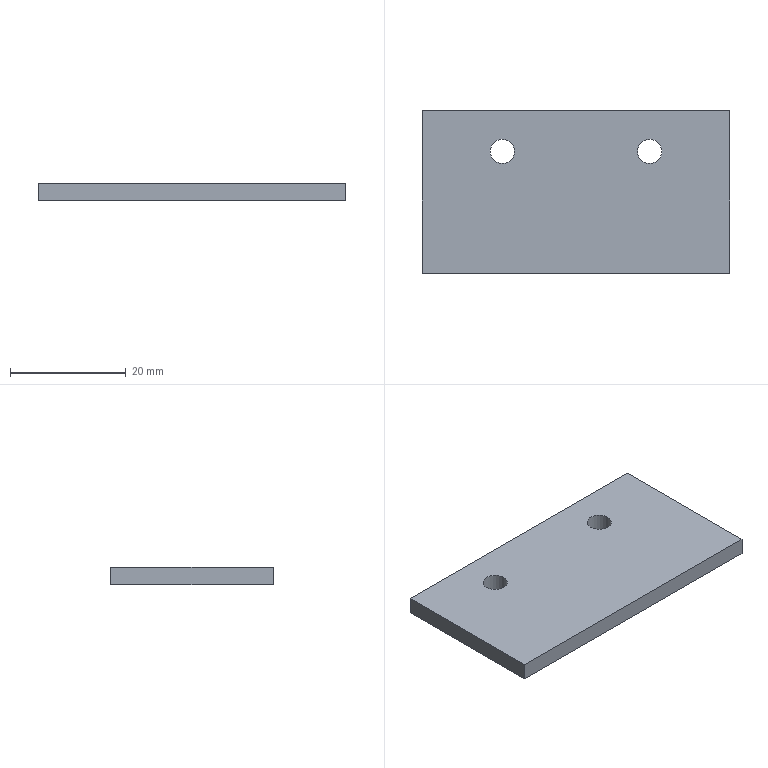Part | NX | features solid 2 | 1 solid | 8 faces | box 53 x 28 x 3 mm | volume 4369 mm3 | plane 6 | cylinder 2 | commonest cylinder face diameters 4.2 x2
STEP:
#1=CARTESIAN_POINT('',(237.929,-475.45,98.));
#2=VERTEX_POINT('',#1);
#3=CARTESIAN_POINT('',(237.929,-503.45,98.));
#4=VERTEX_POINT('',#3);
#5=CARTESIAN_POINT('',(237.929,-475.45,98.));
#6=DIRECTION('',(0.,-1.,0.));
#7=VECTOR('',#6,1000.);
#8=LINE('',#5,#7);
#9=EDGE_CURVE('',#2,#4,#8,.T.);
#10=ORIENTED_EDGE('',*,*,#9,.T.);
#11=CARTESIAN_POINT('',(237.929,-503.45,101.));
#12=VERTEX_POINT('',#11);
#13=CARTESIAN_POINT('',(237.929,-503.45,101.));
#14=DIRECTION('',(0.,0.,-1.));
#15=VECTOR('',#14,1000.);
#16=LINE('',#13,#15);
#17=EDGE_CURVE('',#12,#4,#16,.T.);
#18=ORIENTED_EDGE('',*,*,#17,.F.);
#19=CARTESIAN_POINT('',(237.929,-475.45,101.));
#20=VERTEX_POINT('',#19);
#21=CARTESIAN_POINT('',(237.929,-475.45,101.));
#22=DIRECTION('',(0.,-1.,0.));
#23=VECTOR('',#22,1000.);
#24=LINE('',#21,#23);
#25=EDGE_CURVE('',#20,#12,#24,.T.);
#26=ORIENTED_EDGE('',*,*,#25,.F.);
#27=CARTESIAN_POINT('',(237.929,-475.45,101.));
#28=DIRECTION('',(0.,0.,-1.));
#29=VECTOR('',#28,1000.);
#30=LINE('',#27,#29);
#31=EDGE_CURVE('',#20,#2,#30,.T.);
#32=ORIENTED_EDGE('',*,*,#31,.T.);
#33=EDGE_LOOP('',(#10,#18,#26,#32));
#34=FACE_BOUND('',#33,.T.);
#35=CARTESIAN_POINT('',(237.929,-475.45,101.));
#36=DIRECTION('',(1.,0.,0.));
#37=DIRECTION('',(0.,-1.,0.));
#38=AXIS2_PLACEMENT_3D('',#35,#36,#37);
#39=PLANE('',#38);
#40=ADVANCED_FACE('',(#34),#39,.F.);
#41=CARTESIAN_POINT('',(290.929,-503.45,98.));
#42=VERTEX_POINT('',#41);
#43=CARTESIAN_POINT('',(237.929,-503.45,98.));
#44=DIRECTION('',(1.,0.,0.));
#45=VECTOR('',#44,1000.);
#46=LINE('',#43,#45);
#47=EDGE_CURVE('',#4,#42,#46,.T.);
#48=ORIENTED_EDGE('',*,*,#47,.T.);
#49=CARTESIAN_POINT('',(290.929,-503.45,101.));
#50=VERTEX_POINT('',#49);
#51=CARTESIAN_POINT('',(290.929,-503.45,101.));
#52=DIRECTION('',(0.,0.,-1.));
#53=VECTOR('',#52,1000.);
#54=LINE('',#51,#53);
#55=EDGE_CURVE('',#50,#42,#54,.T.);
#56=ORIENTED_EDGE('',*,*,#55,.F.);
#57=CARTESIAN_POINT('',(237.929,-503.45,101.));
#58=DIRECTION('',(1.,0.,0.));
#59=VECTOR('',#58,1000.);
#60=LINE('',#57,#59);
#61=EDGE_CURVE('',#12,#50,#60,.T.);
#62=ORIENTED_EDGE('',*,*,#61,.F.);
#63=ORIENTED_EDGE('',*,*,#17,.T.);
#64=EDGE_LOOP('',(#48,#56,#62,#63));
#65=FACE_BOUND('',#64,.T.);
#66=CARTESIAN_POINT('',(237.929,-503.45,101.));
#67=DIRECTION('',(0.,1.,0.));
#68=DIRECTION('',(1.,0.,0.));
#69=AXIS2_PLACEMENT_3D('',#66,#67,#68);
#70=PLANE('',#69);
#71=ADVANCED_FACE('',(#65),#70,.F.);
#72=CARTESIAN_POINT('',(290.929,-475.45,98.));
#73=VERTEX_POINT('',#72);
#74=CARTESIAN_POINT('',(290.929,-503.45,98.));
#75=DIRECTION('',(0.,1.,0.));
#76=VECTOR('',#75,1000.);
#77=LINE('',#74,#76);
#78=EDGE_CURVE('',#42,#73,#77,.T.);
#79=ORIENTED_EDGE('',*,*,#78,.T.);
#80=CARTESIAN_POINT('',(290.929,-475.45,101.));
#81=VERTEX_POINT('',#80);
#82=CARTESIAN_POINT('',(290.929,-475.45,101.));
#83=DIRECTION('',(0.,0.,-1.));
#84=VECTOR('',#83,1000.);
#85=LINE('',#82,#84);
#86=EDGE_CURVE('',#81,#73,#85,.T.);
#87=ORIENTED_EDGE('',*,*,#86,.F.);
#88=CARTESIAN_POINT('',(290.929,-503.45,101.));
#89=DIRECTION('',(0.,1.,0.));
#90=VECTOR('',#89,1000.);
#91=LINE('',#88,#90);
#92=EDGE_CURVE('',#50,#81,#91,.T.);
#93=ORIENTED_EDGE('',*,*,#92,.F.);
#94=ORIENTED_EDGE('',*,*,#55,.T.);
#95=EDGE_LOOP('',(#79,#87,#93,#94));
#96=FACE_BOUND('',#95,.T.);
#97=CARTESIAN_POINT('',(290.929,-503.45,101.));
#98=DIRECTION('',(-1.,0.,0.));
#99=DIRECTION('',(0.,1.,0.));
#100=AXIS2_PLACEMENT_3D('',#97,#98,#99);
#101=PLANE('',#100);
#102=ADVANCED_FACE('',(#96),#101,.F.);
#103=CARTESIAN_POINT('',(249.629,-482.45,98.));
#104=VERTEX_POINT('',#103);
#105=CARTESIAN_POINT('',(251.729,-482.45,98.));
#106=DIRECTION('',(0.,0.,1.));
#107=DIRECTION('',(-1.,0.,0.));
#108=AXIS2_PLACEMENT_3D('',#105,#106,#107);
#109=CIRCLE('',#108,2.1);
#110=EDGE_CURVE('',#104,#104,#109,.T.);
#111=ORIENTED_EDGE('',*,*,#110,.F.);
#112=EDGE_LOOP('',(#111));
#113=FACE_BOUND('',#112,.T.);
#114=CARTESIAN_POINT('',(249.629,-482.45,101.));
#115=VERTEX_POINT('',#114);
#116=CARTESIAN_POINT('',(251.729,-482.45,101.));
#117=DIRECTION('',(0.,0.,1.));
#118=DIRECTION('',(-1.,0.,0.));
#119=AXIS2_PLACEMENT_3D('',#116,#117,#118);
#120=CIRCLE('',#119,2.1);
#121=EDGE_CURVE('',#115,#115,#120,.T.);
#122=ORIENTED_EDGE('',*,*,#121,.T.);
#123=EDGE_LOOP('',(#122));
#124=FACE_BOUND('',#123,.T.);
#125=CARTESIAN_POINT('',(251.729,-482.45,101.));
#126=DIRECTION('',(0.,0.,-1.));
#127=DIRECTION('',(0.,-1.,0.));
#128=AXIS2_PLACEMENT_3D('',#125,#126,#127);
#129=CYLINDRICAL_SURFACE('',#128,2.1);
#130=ADVANCED_FACE('',(#113,#124),#129,.F.);
#131=CARTESIAN_POINT('',(290.929,-475.45,98.));
#132=DIRECTION('',(-1.,0.,0.));
#133=VECTOR('',#132,1000.);
#134=LINE('',#131,#133);
#135=EDGE_CURVE('',#73,#2,#134,.T.);
#136=ORIENTED_EDGE('',*,*,#135,.T.);
#137=ORIENTED_EDGE('',*,*,#31,.F.);
#138=CARTESIAN_POINT('',(290.929,-475.45,101.));
#139=DIRECTION('',(-1.,0.,0.));
#140=VECTOR('',#139,1000.);
#141=LINE('',#138,#140);
#142=EDGE_CURVE('',#81,#20,#141,.T.);
#143=ORIENTED_EDGE('',*,*,#142,.F.);
#144=ORIENTED_EDGE('',*,*,#86,.T.);
#145=EDGE_LOOP('',(#136,#137,#143,#144));
#146=FACE_BOUND('',#145,.T.);
#147=CARTESIAN_POINT('',(290.929,-475.45,101.));
#148=DIRECTION('',(0.,-1.,0.));
#149=DIRECTION('',(-1.,0.,0.));
#150=AXIS2_PLACEMENT_3D('',#147,#148,#149);
#151=PLANE('',#150);
#152=ADVANCED_FACE('',(#146),#151,.F.);
#153=CARTESIAN_POINT('',(275.029,-482.45,98.));
#154=VERTEX_POINT('',#153);
#155=CARTESIAN_POINT('',(277.129,-482.45,98.));
#156=DIRECTION('',(0.,0.,1.));
#157=DIRECTION('',(-1.,0.,0.));
#158=AXIS2_PLACEMENT_3D('',#155,#156,#157);
#159=CIRCLE('',#158,2.1);
#160=EDGE_CURVE('',#154,#154,#159,.T.);
#161=ORIENTED_EDGE('',*,*,#160,.F.);
#162=EDGE_LOOP('',(#161));
#163=FACE_BOUND('',#162,.T.);
#164=CARTESIAN_POINT('',(275.029,-482.45,101.));
#165=VERTEX_POINT('',#164);
#166=CARTESIAN_POINT('',(277.129,-482.45,101.));
#167=DIRECTION('',(0.,0.,1.));
#168=DIRECTION('',(-1.,0.,0.));
#169=AXIS2_PLACEMENT_3D('',#166,#167,#168);
#170=CIRCLE('',#169,2.1);
#171=EDGE_CURVE('',#165,#165,#170,.T.);
#172=ORIENTED_EDGE('',*,*,#171,.T.);
#173=EDGE_LOOP('',(#172));
#174=FACE_BOUND('',#173,.T.);
#175=CARTESIAN_POINT('',(277.129,-482.45,101.));
#176=DIRECTION('',(0.,0.,-1.));
#177=DIRECTION('',(0.,-1.,0.));
#178=AXIS2_PLACEMENT_3D('',#175,#176,#177);
#179=CYLINDRICAL_SURFACE('',#178,2.1);
#180=ADVANCED_FACE('',(#163,#174),#179,.F.);
#181=ORIENTED_EDGE('',*,*,#25,.T.);
#182=ORIENTED_EDGE('',*,*,#61,.T.);
#183=ORIENTED_EDGE('',*,*,#92,.T.);
#184=ORIENTED_EDGE('',*,*,#142,.T.);
#185=EDGE_LOOP('',(#181,#182,#183,#184));
#186=FACE_BOUND('',#185,.T.);
#187=ORIENTED_EDGE('',*,*,#121,.F.);
#188=EDGE_LOOP('',(#187));
#189=FACE_BOUND('',#188,.T.);
#190=ORIENTED_EDGE('',*,*,#171,.F.);
#191=EDGE_LOOP('',(#190));
#192=FACE_BOUND('',#191,.T.);
#193=CARTESIAN_POINT('',(237.929,-503.45,101.));
#194=DIRECTION('',(0.,0.,1.));
#195=DIRECTION('',(0.,1.,0.));
#196=AXIS2_PLACEMENT_3D('',#193,#194,#195);
#197=PLANE('',#196);
#198=ADVANCED_FACE('',(#186,#189,#192),#197,.T.);
#199=ORIENTED_EDGE('',*,*,#9,.F.);
#200=ORIENTED_EDGE('',*,*,#135,.F.);
#201=ORIENTED_EDGE('',*,*,#78,.F.);
#202=ORIENTED_EDGE('',*,*,#47,.F.);
#203=EDGE_LOOP('',(#199,#200,#201,#202));
#204=FACE_BOUND('',#203,.T.);
#205=ORIENTED_EDGE('',*,*,#110,.T.);
#206=EDGE_LOOP('',(#205));
#207=FACE_BOUND('',#206,.T.);
#208=ORIENTED_EDGE('',*,*,#160,.T.);
#209=EDGE_LOOP('',(#208));
#210=FACE_BOUND('',#209,.T.);
#211=CARTESIAN_POINT('',(237.929,-503.45,98.));
#212=DIRECTION('',(0.,0.,1.));
#213=DIRECTION('',(0.,1.,0.));
#214=AXIS2_PLACEMENT_3D('',#211,#212,#213);
#215=PLANE('',#214);
#216=ADVANCED_FACE('',(#204,#207,#210),#215,.F.);
#217=CLOSED_SHELL('',(#40,#71,#102,#130,#152,#180,#198,#216));
#218=MANIFOLD_SOLID_BREP('',#217);
#219=(LENGTH_UNIT()NAMED_UNIT(*)SI_UNIT(.MILLI.,.METRE.));
#220=UNCERTAINTY_MEASURE_WITH_UNIT(LENGTH_MEASURE(0.00001),#219,'','');
#221=(NAMED_UNIT(*)PLANE_ANGLE_UNIT()SI_UNIT($,.RADIAN.));
#222=(NAMED_UNIT(*)SI_UNIT($,.STERADIAN.)SOLID_ANGLE_UNIT());
#223=(GEOMETRIC_REPRESENTATION_CONTEXT(3)GLOBAL_UNCERTAINTY_ASSIGNED_CONTEXT((#220))GLOBAL_UNIT_ASSIGNED_CONTEXT((#219,#221,#222))REPRESENTATION_CONTEXT('',''));
#224=ADVANCED_BREP_SHAPE_REPRESENTATION('',(#218),#223);